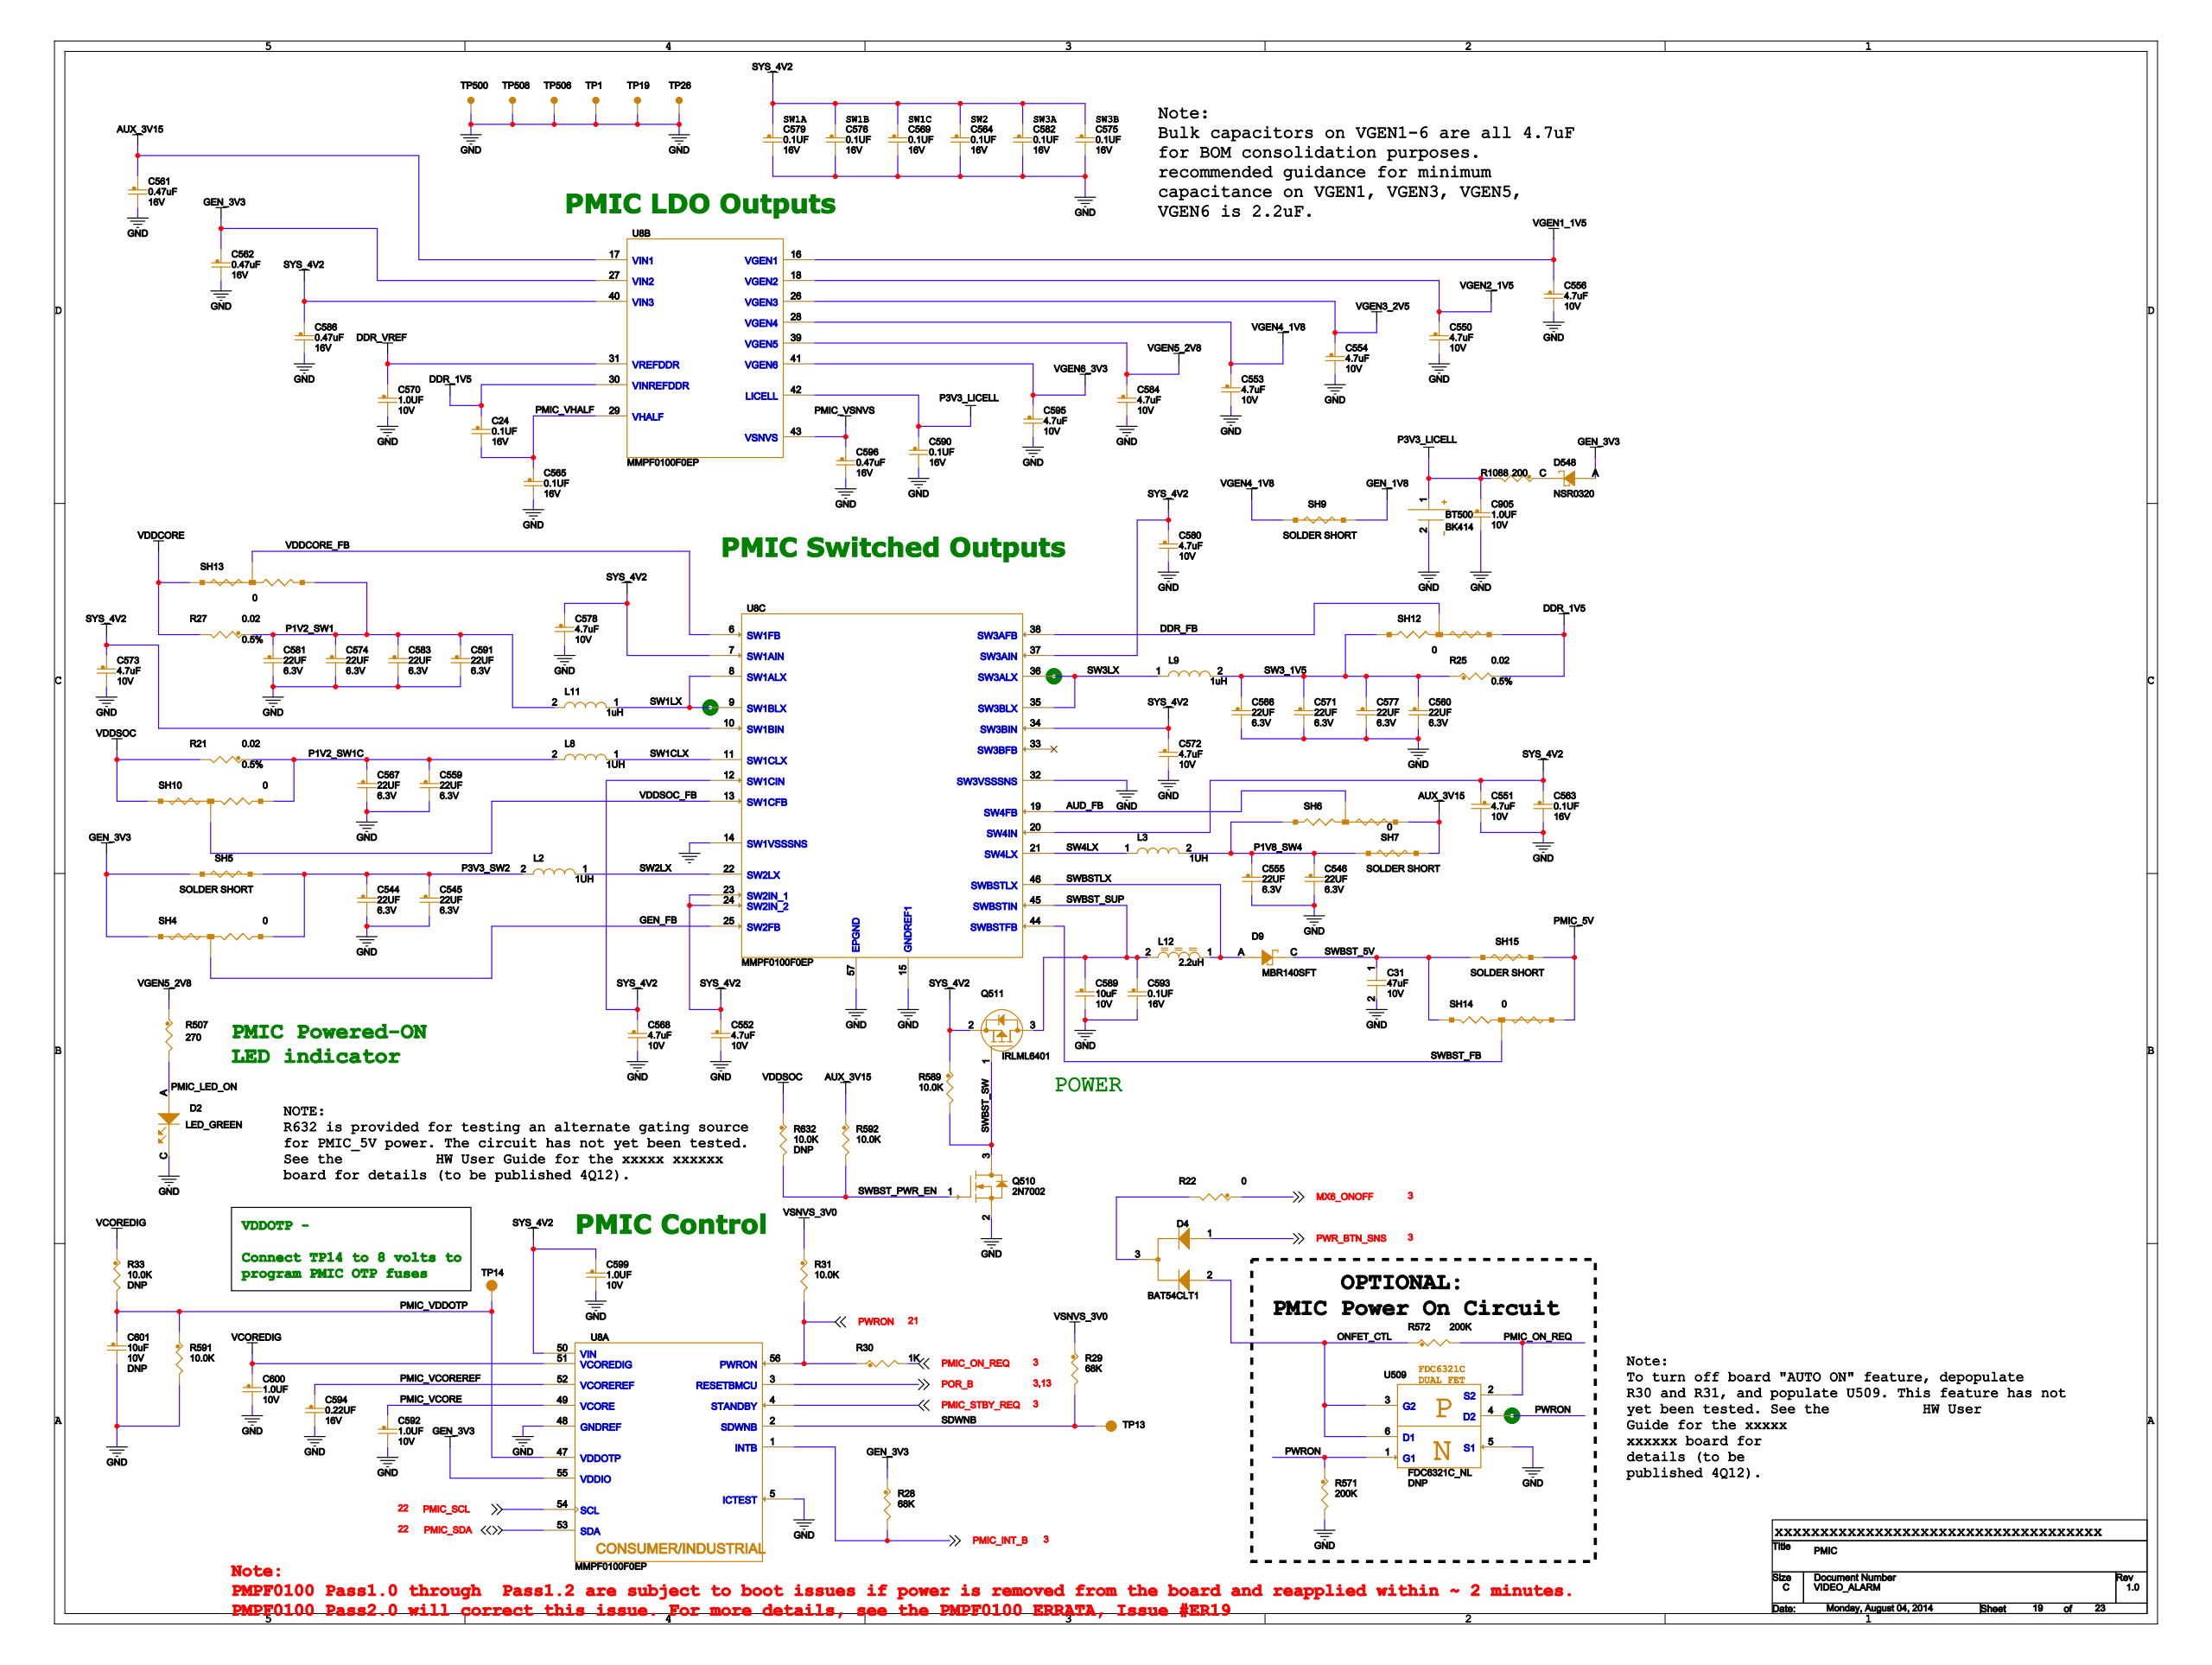Circuit board | Cadence Allegro | 994 parts | 728 nets | one sheet of the schematic
Parts on this sheet (reference | value | footprint):
BT500 | BK414 | BATT_RETAINER_5P08X5P3
C24 | 0.1UF | 0402_CC
C31 | 47uF | 1206_CC
C544 | 22UF | 0603_CC
C545 | 22UF | 0603_CC
C546 | 22UF | 0603_CC
C550 | 4.7uF | 0603_CC
C551 | 4.7uF | 0603_CC
C552 | 4.7uF | 0603_CC
C553 | 4.7uF | 0603_CC
C554 | 4.7uF | 0603_CC
C555 | 22UF | 0603_CC
C556 | 4.7uF | 0603_CC
C559 | 22UF | 0603_CC
C560 | 22UF | 0603_CC
C561 | 0.47uF | 0402_CC
C562 | 0.47uF | 0402_CC
C563 | 0.1UF | 0402_CC
C564 | 0.1UF | 0402_CC
C565 | 0.1UF | 0402_CC
C566 | 22UF | 0603_CC
C567 | 22UF | 0603_CC
C568 | 4.7uF | 0603_CC
C569 | 0.1UF | 0402_CC
C570 | 1.0UF | 0402_CC
C571 | 22UF | 0603_CC
C572 | 4.7uF | 0603_CC
C573 | 4.7uF | 0603_CC
C574 | 22UF | 0603_CC
C575 | 0.1UF | 0402_CC
C576 | 0.1UF | 0402_CC
C577 | 22UF | 0603_CC
C578 | 4.7uF | 0603_CC
C579 | 0.1UF | 0402_CC
C580 | 4.7uF | 0603_CC
C581 | 22UF | 0603_CC
C582 | 0.1UF | 0402_CC
C583 | 22UF | 0603_CC
C584 | 4.7uF | 0603_CC
C586 | 0.47uF | 0402_CC
C589 | 10uF | 0603_CC
C590 | 0.1UF | 0402_CC
C591 | 22UF | 0603_CC
C592 | 1.0UF | 0402_CC
C593 | 0.1UF | 0402_CC
C594 | 0.22UF | 0402_CC
C595 | 4.7uF | 0603_CC
C596 | 0.47uF | 0402_CC
C599 | 1.0UF | 0402_CC
C600 | 1.0UF | 0402_CC
C601 | 10uF | 0603_CC
C905 | 1.0UF | 0402_CC
D2 | LED_GREEN | LED_0603
D4 | BAT54CLT1 | SOT23_A
D9 | MBR140SFT | SOD123LF
D548 | NSR0320 | SOD323
L2 | 1UH | IND_VLS252010
L3 | 1UH | IND_VLS252010
L8 | 1UH | IND_VLS252010
L9 | 1uH | IND_5015
L11 | 1uH | IND_5015
L12 | 2.2uH | IND_LPS4018
Q510 | 2N7002 | SOT23
Q511 | IRLML6401 | SOT-23
R21 | 0.02 | 0805_CC
R25 | 0.02 | 0805_CC
R27 | 0.02 | 0805_CC
R28 | 68K | 0402_CC
R29 | 68K | 0402_CC
R30 | 1K | 0201_CC
R31 | 10.0K | 0402_CC
R33 | 10.0K | 0402_CC
R507 | 270 | 0402_CC
R571 | 200K | 0603_CC
R572 | 200K | 0603_CC
R589 | 10.0K | 0402_CC
R591 | 10.0K | 0402_CC
R592 | 10.0K | 0402_CC
R632 | 10.0K | 0402_CC
R1088 | 200 | 0402_CC
SH4 | 0 | SH0603-X2_PIN1TO2
SH5 | SOLDER SHORT | SH0805_40
SH6 | 0 | SH0603-X2_PIN1TO2
SH7 | SOLDER SHORT | SH0805_40
SH9 | SOLDER SHORT | SH0805_40
SH10 | 0 | SH0603-X2_PIN1TO2
SH12 | 0 | SH0603-X2_PIN1TO2
SH13 | 0 | SH0603-X2_PIN1TO2
SH14 | 0 | SH0603-X2_PIN1TO2
SH15 | SOLDER SHORT | SH0805_40
TP1 | TEST POINT | C035S
TP13 | TPAD_020 | TPAD_020
TP14 | TPAD_020 | TPAD_020
TP19 | TEST POINT | C035S
TP26 | TEST POINT | C035S
TP500 | TEST POINT | C035S
TP506 | TEST POINT | C035S
TP508 | TEST POINT | C035S
U8 | MMPF0100F0EP | QFN56_0P5_8X8_EP4P5
U509 | FDC6321C_NL | SOT23-6
Nets of these parts (net: part-pin ...):
GND: BT500-2 C31-2 C544-2 C545-2 C546-2 C550-2 C551-2 C552-2 C553-2 C554-2 C555-2 C556-2 C559-2 C560-2 C561-2 C562-2 C563-2 C564-2 C565-2 C566-2 C567-2 C568-2 C569-2 C570-2 C571-2 C572-2 C573-2 C574-2 C575-2 C576-2 C577-2 C578-2 C579-2 C580-2 C581-2 C582-2 C583-2 C584-2 C586-2 C589-2 C590-2 C591-2 C592-2 C593-2 C594-2 C595-2 C596-2 C599-2 C600-2 C601-2 C905-2 D2-C Q510-2 R571-2 R591-2 TP1-1 TP19-1 TP26-1 TP500-1 TP506-1 TP508-1 U509-5 U8-5 U8-14 U8-15 U8-32 U8-48 U8-57
PMIC_INT_B: R28-2 U8-1
PWRON: R30-1 R31-2 R571-1 U509-1 U509-4 U8-56
POR_B: U8-3
PMIC_SCL: U8-54
PMIC_SDA: U8-53
SDWNB: R29-2 TP13-1 U8-2
PMIC_STBY_REQ: U8-4
PMIC_VCORE: C592-1 U8-49
VCOREDIG: C600-1 R33-1 U8-51
PMIC_VCOREREF: C594-1 U8-52
GEN_3V3: C562-1 D548-A R28-1 SH4-1 SH5-2 U8-27 U8-55
PMIC_VDDOTP: C601-1 R33-2 R591-1 TP14-1 U8-47
SYS_4V2: C551-1 C552-1 C563-1 C564-1 C568-1 C569-1 C572-1 C573-1 C575-1 C576-1 C578-1 C579-1 C580-1 C582-1 C586-1 C599-1 Q511-2 R589-1 U8-7 U8-10 U8-12 U8-20 U8-23 U8-24 U8-34 U8-37 U8-40 U8-50
P3V3_LICELL: BT500-1 C590-1 C905-1 R1088-2 U8-42
VGEN1_1V5: C556-1 U8-16
VGEN2_1V5: C550-1 U8-18
VGEN3_2V5: C554-1 U8-26
VGEN4_1V8: C553-1 SH9-2 U8-28
VGEN5_2V8: C584-1 R507-1 U8-39
VGEN6_3V3: C595-1 U8-41
PMIC_VHALF: C24-2 C565-1 U8-29
AUX_3V15: C561-1 R592-1 SH6-1 SH7-1 U8-17
DDR_1V5: C24-1 R25-2 SH12-1 U8-30
DDR_VREF: C570-1 U8-31
PMIC_VSNVS: C596-1 U8-43
SW1LX: L11-1 U8-8 U8-9
VDDSOC_FB: SH10-2 U8-13
SW1CLX: L8-1 U8-11
VDDCORE_FB: SH13-2 U8-6
GEN_FB: SH4-2 U8-25
SW2LX: L2-1 U8-22
DDR_FB: SH12-2 U8-38
SW3LX: L9-1 U8-35 U8-36
AUD_FB: SH6-2 U8-19
SW4LX: L3-1 U8-21
SWBST_FB: SH14-2 U8-44
SWBST_SUP: C589-1 C593-1 L12-2 Q511-3 U8-45
SWBSTLX: D9-A L12-1 U8-46
GEN_1V8: SH9-1
P1V8_SW4: C546-1 C555-1 L3-2 SH6-3 SH7-2
P3V3_SW2: C544-1 C545-1 L2-2 SH4-3 SH5-1
PMIC_5V: SH14-1 SH15-1
SWBST_5V: C31-1 D9-C SH14-3 SH15-2
VDDCORE: R27-2 SH13-1
P1V2_SW1: C574-1 C581-1 C583-1 C591-1 L11-2 R27-1 SH13-3
SW3_1V5: C560-1 C566-1 C571-1 C577-1 L9-2 R25-1 SH12-3
VDDSOC: R21-2 R632-1 SH10-1
P1V2_SW1C: C559-1 C567-1 L8-2 R21-1 SH10-3
PMIC_LED_ON: D2-A R507-2
PMIC_ON_REQ: R30-2 R572-2 U509-2
VSNVS_3V0: R29-1 R31-1
ONFET_CTL: D4-2 R572-1 U509-3 U509-6
PWR_BTN_SNS: D4-1
N231582011: D548-C R1088-1
N23053679: D4-3
SWBST_PWR_EN: Q510-1 R592-2 R632-2
SWBST_SW: Q510-3 Q511-1 R589-2